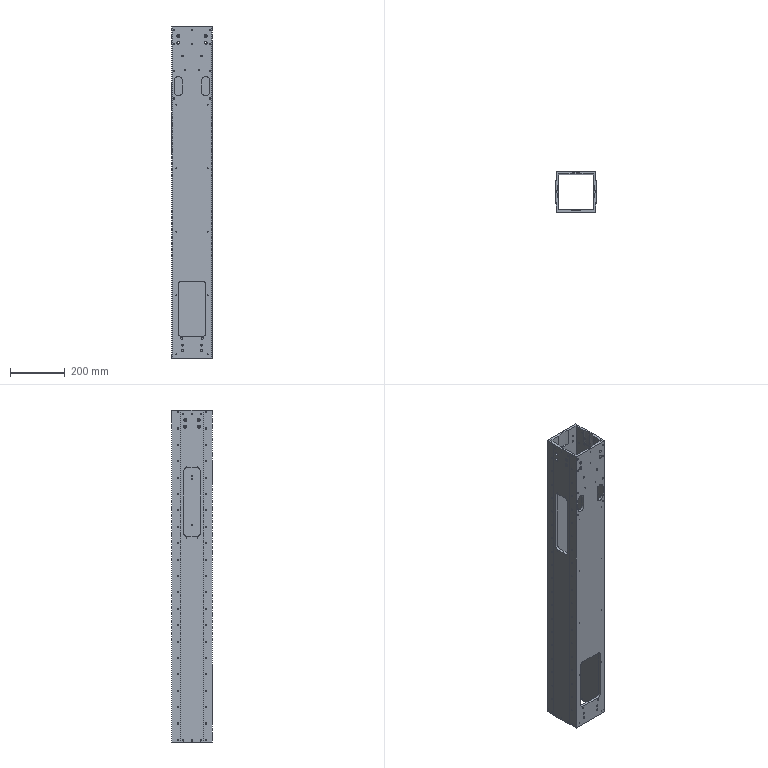Part | SolidWorks | features HoleWzd 14, ICE 3, Cut 2, Fillet 2, Extrusion 1 | 1 solid | 441 faces | box 150 x 150 x 1215 mm | volume 6013792 mm3 | cylinder 369 | plane 48 | cone 24 | commonest cylinder face diameters 4.2 x188 5 x48 3.3 x34 6.6 x32 11 x32 6.8 x16